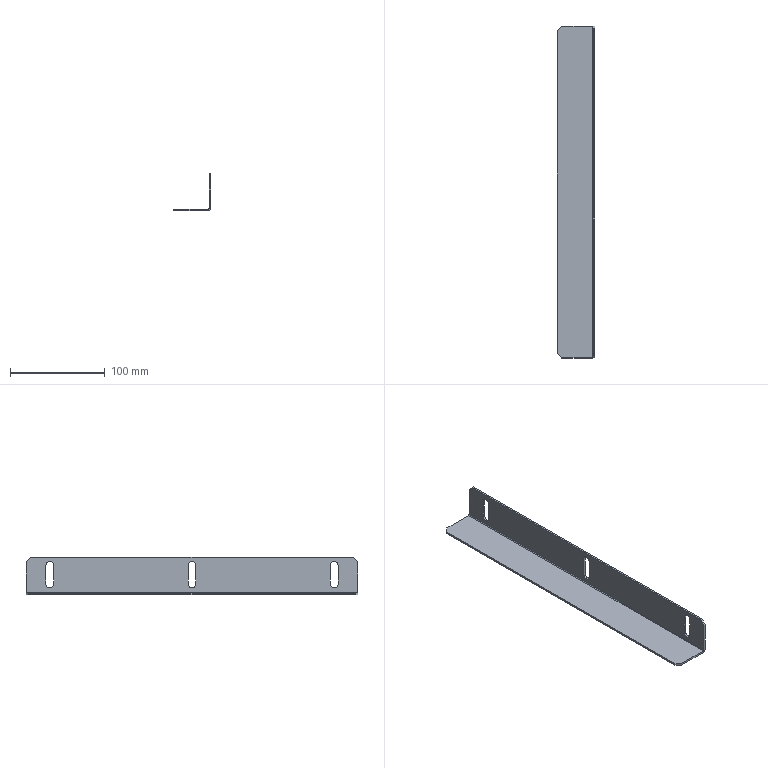Part | SolidWorks | features BreakCorner 1, EdgeFlange 1, FlatPattern 1, HoleWzd 1, SMBaseFlange 1, SheetMetal 1 | 1 solid | 33 faces | box 40 x 350 x 40 mm | volume 52717 mm3 | plane 22 | cylinder 11 | commonest cylinder face diameters 8 x9 1.473 x1 5.473 x1
STEP:
#1=CARTESIAN_POINT('',(20.,154.,29.368));
#2=VERTEX_POINT('',#1);
#3=CARTESIAN_POINT('',(20.,150.,33.368));
#4=VERTEX_POINT('',#3);
#5=CARTESIAN_POINT('',(20.,150.,29.368));
#6=DIRECTION('',(1.,0.,0.));
#7=DIRECTION('',(0.,0.,-1.));
#8=AXIS2_PLACEMENT_3D('',#5,#6,#7);
#9=CIRCLE('',#8,4.);
#10=EDGE_CURVE('',#2,#4,#9,.T.);
#11=ORIENTED_EDGE('',*,*,#10,.T.);
#12=CARTESIAN_POINT('',(18.,150.,33.368));
#13=VERTEX_POINT('',#12);
#14=CARTESIAN_POINT('',(18.,150.,33.368));
#15=DIRECTION('',(-1.,0.,0.));
#16=VECTOR('',#15,1000.);
#17=LINE('',#14,#16);
#18=EDGE_CURVE('',#4,#13,#17,.T.);
#19=ORIENTED_EDGE('',*,*,#18,.T.);
#20=CARTESIAN_POINT('',(18.,154.,29.368));
#21=VERTEX_POINT('',#20);
#22=CARTESIAN_POINT('',(18.,150.,29.368));
#23=DIRECTION('',(-1.,0.,0.));
#24=DIRECTION('',(0.,0.,1.));
#25=AXIS2_PLACEMENT_3D('',#22,#23,#24);
#26=CIRCLE('',#25,4.);
#27=EDGE_CURVE('',#13,#21,#26,.T.);
#28=ORIENTED_EDGE('',*,*,#27,.T.);
#29=CARTESIAN_POINT('',(20.001,154.,29.368));
#30=DIRECTION('',(1.,0.,0.));
#31=VECTOR('',#30,1000.);
#32=LINE('',#29,#31);
#33=EDGE_CURVE('',#21,#2,#32,.T.);
#34=ORIENTED_EDGE('',*,*,#33,.T.);
#35=EDGE_LOOP('',(#11,#19,#28,#34));
#36=FACE_OUTER_BOUND('',#35,.T.);
#37=CARTESIAN_POINT('',(18.,150.,29.368));
#38=DIRECTION('',(-1.,0.,0.));
#39=DIRECTION('',(0.,0.,1.));
#40=AXIS2_PLACEMENT_3D('',#37,#38,#39);
#41=CYLINDRICAL_SURFACE('',#40,4.);
#42=ADVANCED_FACE('',(#36),#41,.F.);
#43=CARTESIAN_POINT('',(20.,4.,29.368));
#44=VERTEX_POINT('',#43);
#45=CARTESIAN_POINT('',(20.,0.,33.368));
#46=VERTEX_POINT('',#45);
#47=CARTESIAN_POINT('',(20.,0.,29.368));
#48=DIRECTION('',(1.,0.,0.));
#49=DIRECTION('',(0.,0.,-1.));
#50=AXIS2_PLACEMENT_3D('',#47,#48,#49);
#51=CIRCLE('',#50,4.);
#52=EDGE_CURVE('',#44,#46,#51,.T.);
#53=ORIENTED_EDGE('',*,*,#52,.T.);
#54=CARTESIAN_POINT('',(18.,0.,33.368));
#55=VERTEX_POINT('',#54);
#56=CARTESIAN_POINT('',(18.,0.,33.368));
#57=DIRECTION('',(-1.,0.,0.));
#58=VECTOR('',#57,1000.);
#59=LINE('',#56,#58);
#60=EDGE_CURVE('',#46,#55,#59,.T.);
#61=ORIENTED_EDGE('',*,*,#60,.T.);
#62=CARTESIAN_POINT('',(18.,4.,29.368));
#63=VERTEX_POINT('',#62);
#64=CARTESIAN_POINT('',(18.,0.,29.368));
#65=DIRECTION('',(-1.,0.,0.));
#66=DIRECTION('',(0.,0.,1.));
#67=AXIS2_PLACEMENT_3D('',#64,#65,#66);
#68=CIRCLE('',#67,4.);
#69=EDGE_CURVE('',#55,#63,#68,.T.);
#70=ORIENTED_EDGE('',*,*,#69,.T.);
#71=CARTESIAN_POINT('',(20.001,4.,29.368));
#72=DIRECTION('',(1.,0.,0.));
#73=VECTOR('',#72,1000.);
#74=LINE('',#71,#73);
#75=EDGE_CURVE('',#63,#44,#74,.T.);
#76=ORIENTED_EDGE('',*,*,#75,.T.);
#77=EDGE_LOOP('',(#53,#61,#70,#76));
#78=FACE_OUTER_BOUND('',#77,.T.);
#79=CARTESIAN_POINT('',(18.,0.,29.368));
#80=DIRECTION('',(-1.,0.,0.));
#81=DIRECTION('',(0.,0.,1.));
#82=AXIS2_PLACEMENT_3D('',#79,#80,#81);
#83=CYLINDRICAL_SURFACE('',#82,4.);
#84=ADVANCED_FACE('',(#78),#83,.F.);
#85=CARTESIAN_POINT('',(20.,-146.,29.368));
#86=VERTEX_POINT('',#85);
#87=CARTESIAN_POINT('',(20.,-150.,33.368));
#88=VERTEX_POINT('',#87);
#89=CARTESIAN_POINT('',(20.,-150.,29.368));
#90=DIRECTION('',(1.,0.,0.));
#91=DIRECTION('',(0.,0.,-1.));
#92=AXIS2_PLACEMENT_3D('',#89,#90,#91);
#93=CIRCLE('',#92,4.);
#94=EDGE_CURVE('',#86,#88,#93,.T.);
#95=ORIENTED_EDGE('',*,*,#94,.T.);
#96=CARTESIAN_POINT('',(18.,-150.,33.368));
#97=VERTEX_POINT('',#96);
#98=CARTESIAN_POINT('',(18.,-150.,33.368));
#99=DIRECTION('',(-1.,0.,0.));
#100=VECTOR('',#99,1000.);
#101=LINE('',#98,#100);
#102=EDGE_CURVE('',#88,#97,#101,.T.);
#103=ORIENTED_EDGE('',*,*,#102,.T.);
#104=CARTESIAN_POINT('',(18.,-146.,29.368));
#105=VERTEX_POINT('',#104);
#106=CARTESIAN_POINT('',(18.,-150.,29.368));
#107=DIRECTION('',(-1.,0.,0.));
#108=DIRECTION('',(0.,0.,1.));
#109=AXIS2_PLACEMENT_3D('',#106,#107,#108);
#110=CIRCLE('',#109,4.);
#111=EDGE_CURVE('',#97,#105,#110,.T.);
#112=ORIENTED_EDGE('',*,*,#111,.T.);
#113=CARTESIAN_POINT('',(20.001,-146.,29.368));
#114=DIRECTION('',(1.,0.,0.));
#115=VECTOR('',#114,1000.);
#116=LINE('',#113,#115);
#117=EDGE_CURVE('',#105,#86,#116,.T.);
#118=ORIENTED_EDGE('',*,*,#117,.T.);
#119=EDGE_LOOP('',(#95,#103,#112,#118));
#120=FACE_OUTER_BOUND('',#119,.T.);
#121=CARTESIAN_POINT('',(18.,-150.,29.368));
#122=DIRECTION('',(-1.,0.,0.));
#123=DIRECTION('',(0.,0.,1.));
#124=AXIS2_PLACEMENT_3D('',#121,#122,#123);
#125=CYLINDRICAL_SURFACE('',#124,4.);
#126=ADVANCED_FACE('',(#120),#125,.F.);
#127=CARTESIAN_POINT('',(20.,175.,33.));
#128=VERTEX_POINT('',#127);
#129=CARTESIAN_POINT('',(20.,175.,0.7366));
#130=VERTEX_POINT('',#129);
#131=CARTESIAN_POINT('',(20.,175.,0.));
#132=DIRECTION('',(0.,0.,-1.));
#133=VECTOR('',#132,1000.);
#134=LINE('',#131,#133);
#135=EDGE_CURVE('',#128,#130,#134,.T.);
#136=ORIENTED_EDGE('',*,*,#135,.F.);
#137=CARTESIAN_POINT('',(20.,170.,38.));
#138=VERTEX_POINT('',#137);
#139=CARTESIAN_POINT('',(20.,104.,104.));
#140=DIRECTION('',(0.,-0.7071,0.7071));
#141=VECTOR('',#140,1000.);
#142=LINE('',#139,#141);
#143=EDGE_CURVE('',#128,#138,#142,.T.);
#144=ORIENTED_EDGE('',*,*,#143,.T.);
#145=CARTESIAN_POINT('',(20.,-170.,38.));
#146=VERTEX_POINT('',#145);
#147=CARTESIAN_POINT('',(20.,175.,38.));
#148=DIRECTION('',(0.,1.,0.));
#149=VECTOR('',#148,1000.);
#150=LINE('',#147,#149);
#151=EDGE_CURVE('',#146,#138,#150,.T.);
#152=ORIENTED_EDGE('',*,*,#151,.F.);
#153=CARTESIAN_POINT('',(20.,-175.,33.));
#154=VERTEX_POINT('',#153);
#155=CARTESIAN_POINT('',(20.,-104.,104.));
#156=DIRECTION('',(0.,-0.7071,-0.7071));
#157=VECTOR('',#156,1000.);
#158=LINE('',#155,#157);
#159=EDGE_CURVE('',#146,#154,#158,.T.);
#160=ORIENTED_EDGE('',*,*,#159,.T.);
#161=CARTESIAN_POINT('',(20.,-175.,0.7366));
#162=VERTEX_POINT('',#161);
#163=CARTESIAN_POINT('',(20.,-175.,38.));
#164=DIRECTION('',(0.,0.,1.));
#165=VECTOR('',#164,1000.);
#166=LINE('',#163,#165);
#167=EDGE_CURVE('',#162,#154,#166,.T.);
#168=ORIENTED_EDGE('',*,*,#167,.F.);
#169=CARTESIAN_POINT('',(20.,0.,0.7366));
#170=DIRECTION('',(0.,1.,0.));
#171=VECTOR('',#170,1000.);
#172=LINE('',#169,#171);
#173=EDGE_CURVE('',#162,#130,#172,.T.);
#174=ORIENTED_EDGE('',*,*,#173,.T.);
#175=EDGE_LOOP('',(#136,#144,#152,#160,#168,#174));
#176=FACE_OUTER_BOUND('',#175,.T.);
#177=ORIENTED_EDGE('',*,*,#94,.F.);
#178=CARTESIAN_POINT('',(20.,-146.,9.368));
#179=VERTEX_POINT('',#178);
#180=CARTESIAN_POINT('',(20.,-146.,0.));
#181=DIRECTION('',(0.,0.,-1.));
#182=VECTOR('',#181,1000.);
#183=LINE('',#180,#182);
#184=EDGE_CURVE('',#86,#179,#183,.T.);
#185=ORIENTED_EDGE('',*,*,#184,.T.);
#186=CARTESIAN_POINT('',(20.,-154.,9.368));
#187=VERTEX_POINT('',#186);
#188=CARTESIAN_POINT('',(20.,-150.,9.368));
#189=DIRECTION('',(1.,0.,0.));
#190=DIRECTION('',(0.,0.,-1.));
#191=AXIS2_PLACEMENT_3D('',#188,#189,#190);
#192=CIRCLE('',#191,4.);
#193=EDGE_CURVE('',#187,#179,#192,.T.);
#194=ORIENTED_EDGE('',*,*,#193,.F.);
#195=CARTESIAN_POINT('',(20.,-154.,29.368));
#196=VERTEX_POINT('',#195);
#197=CARTESIAN_POINT('',(20.,-154.,0.));
#198=DIRECTION('',(0.,0.,-1.));
#199=VECTOR('',#198,1000.);
#200=LINE('',#197,#199);
#201=EDGE_CURVE('',#196,#187,#200,.T.);
#202=ORIENTED_EDGE('',*,*,#201,.F.);
#203=CARTESIAN_POINT('',(20.,-150.,29.368));
#204=DIRECTION('',(1.,0.,0.));
#205=DIRECTION('',(0.,0.,-1.));
#206=AXIS2_PLACEMENT_3D('',#203,#204,#205);
#207=CIRCLE('',#206,4.);
#208=EDGE_CURVE('',#88,#196,#207,.T.);
#209=ORIENTED_EDGE('',*,*,#208,.F.);
#210=EDGE_LOOP('',(#177,#185,#194,#202,#209));
#211=FACE_BOUND('',#210,.T.);
#212=ORIENTED_EDGE('',*,*,#52,.F.);
#213=CARTESIAN_POINT('',(20.,4.,9.368));
#214=VERTEX_POINT('',#213);
#215=CARTESIAN_POINT('',(20.,4.,0.));
#216=DIRECTION('',(0.,0.,-1.));
#217=VECTOR('',#216,1000.);
#218=LINE('',#215,#217);
#219=EDGE_CURVE('',#44,#214,#218,.T.);
#220=ORIENTED_EDGE('',*,*,#219,.T.);
#221=CARTESIAN_POINT('',(20.,-4.,9.368));
#222=VERTEX_POINT('',#221);
#223=CARTESIAN_POINT('',(20.,0.,9.368));
#224=DIRECTION('',(1.,0.,0.));
#225=DIRECTION('',(0.,0.,-1.));
#226=AXIS2_PLACEMENT_3D('',#223,#224,#225);
#227=CIRCLE('',#226,4.);
#228=EDGE_CURVE('',#222,#214,#227,.T.);
#229=ORIENTED_EDGE('',*,*,#228,.F.);
#230=CARTESIAN_POINT('',(20.,-4.,29.368));
#231=VERTEX_POINT('',#230);
#232=CARTESIAN_POINT('',(20.,-4.,0.));
#233=DIRECTION('',(0.,0.,-1.));
#234=VECTOR('',#233,1000.);
#235=LINE('',#232,#234);
#236=EDGE_CURVE('',#231,#222,#235,.T.);
#237=ORIENTED_EDGE('',*,*,#236,.F.);
#238=CARTESIAN_POINT('',(20.,0.,29.368));
#239=DIRECTION('',(1.,0.,0.));
#240=DIRECTION('',(0.,0.,-1.));
#241=AXIS2_PLACEMENT_3D('',#238,#239,#240);
#242=CIRCLE('',#241,4.);
#243=EDGE_CURVE('',#46,#231,#242,.T.);
#244=ORIENTED_EDGE('',*,*,#243,.F.);
#245=EDGE_LOOP('',(#212,#220,#229,#237,#244));
#246=FACE_BOUND('',#245,.T.);
#247=ORIENTED_EDGE('',*,*,#10,.F.);
#248=CARTESIAN_POINT('',(20.,154.,9.368));
#249=VERTEX_POINT('',#248);
#250=CARTESIAN_POINT('',(20.,154.,0.));
#251=DIRECTION('',(0.,0.,-1.));
#252=VECTOR('',#251,1000.);
#253=LINE('',#250,#252);
#254=EDGE_CURVE('',#2,#249,#253,.T.);
#255=ORIENTED_EDGE('',*,*,#254,.T.);
#256=CARTESIAN_POINT('',(20.,146.,9.368));
#257=VERTEX_POINT('',#256);
#258=CARTESIAN_POINT('',(20.,150.,9.368));
#259=DIRECTION('',(1.,0.,0.));
#260=DIRECTION('',(0.,0.,-1.));
#261=AXIS2_PLACEMENT_3D('',#258,#259,#260);
#262=CIRCLE('',#261,4.);
#263=EDGE_CURVE('',#257,#249,#262,.T.);
#264=ORIENTED_EDGE('',*,*,#263,.F.);
#265=CARTESIAN_POINT('',(20.,146.,29.368));
#266=VERTEX_POINT('',#265);
#267=CARTESIAN_POINT('',(20.,146.,0.));
#268=DIRECTION('',(0.,0.,-1.));
#269=VECTOR('',#268,1000.);
#270=LINE('',#267,#269);
#271=EDGE_CURVE('',#266,#257,#270,.T.);
#272=ORIENTED_EDGE('',*,*,#271,.F.);
#273=CARTESIAN_POINT('',(20.,150.,29.368));
#274=DIRECTION('',(1.,0.,0.));
#275=DIRECTION('',(0.,0.,-1.));
#276=AXIS2_PLACEMENT_3D('',#273,#274,#275);
#277=CIRCLE('',#276,4.);
#278=EDGE_CURVE('',#4,#266,#277,.T.);
#279=ORIENTED_EDGE('',*,*,#278,.F.);
#280=EDGE_LOOP('',(#247,#255,#264,#272,#279));
#281=FACE_BOUND('',#280,.T.);
#282=CARTESIAN_POINT('',(20.,0.,0.));
#283=DIRECTION('',(1.,0.,0.));
#284=DIRECTION('',(0.,0.,-1.));
#285=AXIS2_PLACEMENT_3D('',#282,#283,#284);
#286=PLANE('',#285);
#287=ADVANCED_FACE('',(#176,#211,#246,#281),#286,.T.);
#288=CARTESIAN_POINT('',(18.,154.,9.368));
#289=VERTEX_POINT('',#288);
#290=CARTESIAN_POINT('',(18.,154.,9.368));
#291=DIRECTION('',(0.,0.,1.));
#292=VECTOR('',#291,1000.);
#293=LINE('',#290,#292);
#294=EDGE_CURVE('',#289,#21,#293,.T.);
#295=ORIENTED_EDGE('',*,*,#294,.T.);
#296=ORIENTED_EDGE('',*,*,#27,.F.);
#297=CARTESIAN_POINT('',(18.,146.,29.368));
#298=VERTEX_POINT('',#297);
#299=CARTESIAN_POINT('',(18.,150.,29.368));
#300=DIRECTION('',(-1.,0.,0.));
#301=DIRECTION('',(0.,0.,1.));
#302=AXIS2_PLACEMENT_3D('',#299,#300,#301);
#303=CIRCLE('',#302,4.);
#304=EDGE_CURVE('',#298,#13,#303,.T.);
#305=ORIENTED_EDGE('',*,*,#304,.F.);
#306=CARTESIAN_POINT('',(18.,146.,9.368));
#307=VERTEX_POINT('',#306);
#308=CARTESIAN_POINT('',(18.,146.,9.368));
#309=DIRECTION('',(0.,0.,1.));
#310=VECTOR('',#309,1000.);
#311=LINE('',#308,#310);
#312=EDGE_CURVE('',#307,#298,#311,.T.);
#313=ORIENTED_EDGE('',*,*,#312,.F.);
#314=CARTESIAN_POINT('',(18.,150.,9.368));
#315=DIRECTION('',(-1.,0.,0.));
#316=DIRECTION('',(0.,0.,1.));
#317=AXIS2_PLACEMENT_3D('',#314,#315,#316);
#318=CIRCLE('',#317,4.);
#319=EDGE_CURVE('',#289,#307,#318,.T.);
#320=ORIENTED_EDGE('',*,*,#319,.F.);
#321=EDGE_LOOP('',(#295,#296,#305,#313,#320));
#322=FACE_BOUND('',#321,.T.);
#323=CARTESIAN_POINT('',(18.,-154.,9.368));
#324=VERTEX_POINT('',#323);
#325=CARTESIAN_POINT('',(18.,-154.,29.368));
#326=VERTEX_POINT('',#325);
#327=CARTESIAN_POINT('',(18.,-154.,9.368));
#328=DIRECTION('',(0.,0.,1.));
#329=VECTOR('',#328,1000.);
#330=LINE('',#327,#329);
#331=EDGE_CURVE('',#324,#326,#330,.T.);
#332=ORIENTED_EDGE('',*,*,#331,.F.);
#333=CARTESIAN_POINT('',(18.,-146.,9.368));
#334=VERTEX_POINT('',#333);
#335=CARTESIAN_POINT('',(18.,-150.,9.368));
#336=DIRECTION('',(-1.,0.,0.));
#337=DIRECTION('',(0.,0.,1.));
#338=AXIS2_PLACEMENT_3D('',#335,#336,#337);
#339=CIRCLE('',#338,4.);
#340=EDGE_CURVE('',#334,#324,#339,.T.);
#341=ORIENTED_EDGE('',*,*,#340,.F.);
#342=CARTESIAN_POINT('',(18.,-146.,9.368));
#343=DIRECTION('',(0.,0.,1.));
#344=VECTOR('',#343,1000.);
#345=LINE('',#342,#344);
#346=EDGE_CURVE('',#334,#105,#345,.T.);
#347=ORIENTED_EDGE('',*,*,#346,.T.);
#348=ORIENTED_EDGE('',*,*,#111,.F.);
#349=CARTESIAN_POINT('',(18.,-150.,29.368));
#350=DIRECTION('',(-1.,0.,0.));
#351=DIRECTION('',(0.,0.,1.));
#352=AXIS2_PLACEMENT_3D('',#349,#350,#351);
#353=CIRCLE('',#352,4.);
#354=EDGE_CURVE('',#326,#97,#353,.T.);
#355=ORIENTED_EDGE('',*,*,#354,.F.);
#356=EDGE_LOOP('',(#332,#341,#347,#348,#355));
#357=FACE_BOUND('',#356,.T.);
#358=CARTESIAN_POINT('',(18.,-170.,38.));
#359=VERTEX_POINT('',#358);
#360=CARTESIAN_POINT('',(18.,170.,38.));
#361=VERTEX_POINT('',#360);
#362=CARTESIAN_POINT('',(18.,0.,38.));
#363=DIRECTION('',(0.,1.,0.));
#364=VECTOR('',#363,1000.);
#365=LINE('',#362,#364);
#366=EDGE_CURVE('',#359,#361,#365,.T.);
#367=ORIENTED_EDGE('',*,*,#366,.T.);
#368=CARTESIAN_POINT('',(18.,175.,33.));
#369=VERTEX_POINT('',#368);
#370=CARTESIAN_POINT('',(18.,170.,38.));
#371=DIRECTION('',(0.,0.7071,-0.7071));
#372=VECTOR('',#371,1000.);
#373=LINE('',#370,#372);
#374=EDGE_CURVE('',#361,#369,#373,.T.);
#375=ORIENTED_EDGE('',*,*,#374,.T.);
#376=CARTESIAN_POINT('',(18.,175.,0.7366));
#377=VERTEX_POINT('',#376);
#378=CARTESIAN_POINT('',(18.,175.,0.));
#379=DIRECTION('',(0.,0.,-1.));
#380=VECTOR('',#379,1000.);
#381=LINE('',#378,#380);
#382=EDGE_CURVE('',#369,#377,#381,.T.);
#383=ORIENTED_EDGE('',*,*,#382,.T.);
#384=CARTESIAN_POINT('',(18.,-175.,0.7366));
#385=VERTEX_POINT('',#384);
#386=CARTESIAN_POINT('',(18.,-175.,0.7366));
#387=DIRECTION('',(0.,1.,0.));
#388=VECTOR('',#387,1000.);
#389=LINE('',#386,#388);
#390=EDGE_CURVE('',#385,#377,#389,.T.);
#391=ORIENTED_EDGE('',*,*,#390,.F.);
#392=CARTESIAN_POINT('',(18.,-175.,33.));
#393=VERTEX_POINT('',#392);
#394=CARTESIAN_POINT('',(18.,-175.,0.));
#395=DIRECTION('',(0.,0.,1.));
#396=VECTOR('',#395,1000.);
#397=LINE('',#394,#396);
#398=EDGE_CURVE('',#385,#393,#397,.T.);
#399=ORIENTED_EDGE('',*,*,#398,.T.);
#400=CARTESIAN_POINT('',(18.,-175.,33.));
#401=DIRECTION('',(0.,0.7071,0.7071));
#402=VECTOR('',#401,1000.);
#403=LINE('',#400,#402);
#404=EDGE_CURVE('',#393,#359,#403,.T.);
#405=ORIENTED_EDGE('',*,*,#404,.T.);
#406=EDGE_LOOP('',(#367,#375,#383,#391,#399,#405));
#407=FACE_OUTER_BOUND('',#406,.T.);
#408=CARTESIAN_POINT('',(18.,-4.,9.368));
#409=VERTEX_POINT('',#408);
#410=CARTESIAN_POINT('',(18.,-4.,29.368));
#411=VERTEX_POINT('',#410);
#412=CARTESIAN_POINT('',(18.,-4.,9.368));
#413=DIRECTION('',(0.,0.,1.));
#414=VECTOR('',#413,1000.);
#415=LINE('',#412,#414);
#416=EDGE_CURVE('',#409,#411,#415,.T.);
#417=ORIENTED_EDGE('',*,*,#416,.F.);
#418=CARTESIAN_POINT('',(18.,4.,9.368));
#419=VERTEX_POINT('',#418);
#420=CARTESIAN_POINT('',(18.,0.,9.368));
#421=DIRECTION('',(-1.,0.,0.));
#422=DIRECTION('',(0.,0.,1.));
#423=AXIS2_PLACEMENT_3D('',#420,#421,#422);
#424=CIRCLE('',#423,4.);
#425=EDGE_CURVE('',#419,#409,#424,.T.);
#426=ORIENTED_EDGE('',*,*,#425,.F.);
#427=CARTESIAN_POINT('',(18.,4.,9.368));
#428=DIRECTION('',(0.,0.,1.));
#429=VECTOR('',#428,1000.);
#430=LINE('',#427,#429);
#431=EDGE_CURVE('',#419,#63,#430,.T.);
#432=ORIENTED_EDGE('',*,*,#431,.T.);
#433=ORIENTED_EDGE('',*,*,#69,.F.);
#434=CARTESIAN_POINT('',(18.,0.,29.368));
#435=DIRECTION('',(-1.,0.,0.));
#436=DIRECTION('',(0.,0.,1.));
#437=AXIS2_PLACEMENT_3D('',#434,#435,#436);
#438=CIRCLE('',#437,4.);
#439=EDGE_CURVE('',#411,#55,#438,.T.);
#440=ORIENTED_EDGE('',*,*,#439,.F.);
#441=EDGE_LOOP('',(#417,#426,#432,#433,#440));
#442=FACE_BOUND('',#441,.T.);
#443=CARTESIAN_POINT('',(18.,0.,0.));
#444=DIRECTION('',(1.,0.,0.));
#445=DIRECTION('',(0.,0.,-1.));
#446=AXIS2_PLACEMENT_3D('',#443,#444,#445);
#447=PLANE('',#446);
#448=ADVANCED_FACE('',(#322,#357,#407,#442),#447,.F.);
#449=CARTESIAN_POINT('',(17.263,175.,-2.));
#450=VERTEX_POINT('',#449);
#451=CARTESIAN_POINT('',(-15.,175.,-2.));
#452=VERTEX_POINT('',#451);
#453=CARTESIAN_POINT('',(-20.,175.,-2.));
#454=DIRECTION('',(-1.,0.,0.));
#455=VECTOR('',#454,1000.);
#456=LINE('',#453,#455);
#457=EDGE_CURVE('',#450,#452,#456,.T.);
#458=ORIENTED_EDGE('',*,*,#457,.T.);
#459=CARTESIAN_POINT('',(-15.,175.,0.));
#460=VERTEX_POINT('',#459);
#461=CARTESIAN_POINT('',(-15.,175.,-2.));
#462=DIRECTION('',(0.,0.,1.));
#463=VECTOR('',#462,1000.);
#464=LINE('',#461,#463);
#465=EDGE_CURVE('',#452,#460,#464,.T.);
#466=ORIENTED_EDGE('',*,*,#465,.T.);
#467=CARTESIAN_POINT('',(17.263,175.,0.));
#468=VERTEX_POINT('',#467);
#469=CARTESIAN_POINT('',(-20.,175.,0.));
#470=DIRECTION('',(-1.,0.,0.));
#471=VECTOR('',#470,1000.);
#472=LINE('',#469,#471);
#473=EDGE_CURVE('',#468,#460,#472,.T.);
#474=ORIENTED_EDGE('',*,*,#473,.F.);
#475=CARTESIAN_POINT('',(17.263,175.,0.));
#476=DIRECTION('',(0.,0.,-1.));
#477=VECTOR('',#476,1000.);
#478=LINE('',#475,#477);
#479=EDGE_CURVE('',#468,#450,#478,.T.);
#480=ORIENTED_EDGE('',*,*,#479,.T.);
#481=EDGE_LOOP('',(#458,#466,#474,#480));
#482=FACE_OUTER_BOUND('',#481,.T.);
#483=CARTESIAN_POINT('',(-20.,175.,-2.));
#484=DIRECTION('',(0.,1.,0.));
#485=DIRECTION('',(0.,0.,1.));
#486=AXIS2_PLACEMENT_3D('',#483,#484,#485);
#487=PLANE('',#486);
#488=ADVANCED_FACE('',(#482),#487,.T.);
#489=CARTESIAN_POINT('',(-15.,-175.,-2.));
#490=VERTEX_POINT('',#489);
#491=CARTESIAN_POINT('',(17.263,-175.,-2.));
#492=VERTEX_POINT('',#491);
#493=CARTESIAN_POINT('',(-20.,-175.,-2.));
#494=DIRECTION('',(1.,0.,0.));
#495=VECTOR('',#494,1000.);
#496=LINE('',#493,#495);
#497=EDGE_CURVE('',#490,#492,#496,.T.);
#498=ORIENTED_EDGE('',*,*,#497,.F.);
#499=CARTESIAN_POINT('',(-20.,-170.,-2.));
#500=VERTEX_POINT('',#499);
#501=CARTESIAN_POINT('',(-95.,-95.,-2.));
#502=DIRECTION('',(-0.7071,0.7071,0.));
#503=VECTOR('',#502,1000.);
#504=LINE('',#501,#503);
#505=EDGE_CURVE('',#490,#500,#504,.T.);
#506=ORIENTED_EDGE('',*,*,#505,.T.);
#507=CARTESIAN_POINT('',(-20.,170.,-2.));
#508=VERTEX_POINT('',#507);
#509=CARTESIAN_POINT('',(-20.,-175.,-2.));
#510=DIRECTION('',(0.,-1.,0.));
#511=VECTOR('',#510,1000.);
#512=LINE('',#509,#511);
#513=EDGE_CURVE('',#508,#500,#512,.T.);
#514=ORIENTED_EDGE('',*,*,#513,.F.);
#515=CARTESIAN_POINT('',(-95.,95.,-2.));
#516=DIRECTION('',(0.7071,0.7071,0.));
#517=VECTOR('',#516,1000.);
#518=LINE('',#515,#517);
#519=EDGE_CURVE('',#508,#452,#518,.T.);
#520=ORIENTED_EDGE('',*,*,#519,.T.);
#521=ORIENTED_EDGE('',*,*,#457,.F.);
#522=CARTESIAN_POINT('',(17.263,175.,-2.));
#523=DIRECTION('',(0.,-1.,0.));
#524=VECTOR('',#523,1000.);
#525=LINE('',#522,#524);
#526=EDGE_CURVE('',#450,#492,#525,.T.);
#527=ORIENTED_EDGE('',*,*,#526,.T.);
#528=EDGE_LOOP('',(#498,#506,#514,#520,#521,#527));
#529=FACE_OUTER_BOUND('',#528,.T.);
#530=CARTESIAN_POINT('',(0.,0.,-2.));
#531=DIRECTION('',(0.,0.,-1.));
#532=DIRECTION('',(-1.,0.,0.));
#533=AXIS2_PLACEMENT_3D('',#530,#531,#532);
#534=PLANE('',#533);
#535=ADVANCED_FACE('',(#529),#534,.T.);
#536=CARTESIAN_POINT('',(-20.,170.,0.));
#537=VERTEX_POINT('',#536);
#538=CARTESIAN_POINT('',(-20.,-170.,0.));
#539=VERTEX_POINT('',#538);
#540=CARTESIAN_POINT('',(-20.,-175.,0.));
#541=DIRECTION('',(0.,-1.,0.));
#542=VECTOR('',#541,1000.);
#543=LINE('',#540,#542);
#544=EDGE_CURVE('',#537,#539,#543,.T.);
#545=ORIENTED_EDGE('',*,*,#544,.T.);
#546=CARTESIAN_POINT('',(-15.,-175.,0.));
#547=VERTEX_POINT('',#546);
#548=CARTESIAN_POINT('',(-20.,-170.,0.));
#549=DIRECTION('',(0.7071,-0.7071,0.));
#550=VECTOR('',#549,1000.);
#551=LINE('',#548,#550);
#552=EDGE_CURVE('',#539,#547,#551,.T.);
#553=ORIENTED_EDGE('',*,*,#552,.T.);
#554=CARTESIAN_POINT('',(17.263,-175.,0.));
#555=VERTEX_POINT('',#554);
#556=CARTESIAN_POINT('',(-20.,-175.,0.));
#557=DIRECTION('',(1.,0.,0.));
#558=VECTOR('',#557,1000.);
#559=LINE('',#556,#558);
#560=EDGE_CURVE('',#547,#555,#559,.T.);
#561=ORIENTED_EDGE('',*,*,#560,.T.);
#562=CARTESIAN_POINT('',(17.263,175.,0.));
#563=DIRECTION('',(0.,-1.,0.));
#564=VECTOR('',#563,1000.);
#565=LINE('',#562,#564);
#566=EDGE_CURVE('',#468,#555,#565,.T.);
#567=ORIENTED_EDGE('',*,*,#566,.F.);
#568=ORIENTED_EDGE('',*,*,#473,.T.);
#569=CARTESIAN_POINT('',(-15.,175.,0.));
#570=DIRECTION('',(-0.7071,-0.7071,0.));
#571=VECTOR('',#570,1000.);
#572=LINE('',#569,#571);
#573=EDGE_CURVE('',#460,#537,#572,.T.);
#574=ORIENTED_EDGE('',*,*,#573,.T.);
#575=EDGE_LOOP('',(#545,#553,#561,#567,#568,#574));
#576=FACE_OUTER_BOUND('',#575,.T.);
#577=CARTESIAN_POINT('',(0.,0.,0.));
#578=DIRECTION('',(0.,0.,-1.));
#579=DIRECTION('',(-1.,0.,0.));
#580=AXIS2_PLACEMENT_3D('',#577,#578,#579);
#581=PLANE('',#580);
#582=ADVANCED_FACE('',(#576),#581,.F.);
#583=ORIENTED_EDGE('',*,*,#560,.F.);
#584=CARTESIAN_POINT('',(-15.,-175.,-2.));
#585=DIRECTION('',(0.,0.,-1.));
#586=VECTOR('',#585,1000.);
#587=LINE('',#584,#586);
#588=EDGE_CURVE('',#547,#490,#587,.T.);
#589=ORIENTED_EDGE('',*,*,#588,.T.);
#590=ORIENTED_EDGE('',*,*,#497,.T.);
#591=CARTESIAN_POINT('',(17.263,-175.,0.));
#592=DIRECTION('',(0.,0.,-1.));
#593=VECTOR('',#592,1000.);
#594=LINE('',#591,#593);
#595=EDGE_CURVE('',#555,#492,#594,.T.);
#596=ORIENTED_EDGE('',*,*,#595,.F.);
#597=EDGE_LOOP('',(#583,#589,#590,#596));
#598=FACE_OUTER_BOUND('',#597,.T.);
#599=CARTESIAN_POINT('',(-20.,-175.,-2.));
#600=DIRECTION('',(0.,-1.,0.));
#601=DIRECTION('',(0.,0.,-1.));
#602=AXIS2_PLACEMENT_3D('',#599,#600,#601);
#603=PLANE('',#602);
#604=ADVANCED_FACE('',(#598),#603,.T.);
#605=ORIENTED_EDGE('',*,*,#513,.T.);
#606=CARTESIAN_POINT('',(-20.,-170.,-2.));
#607=DIRECTION('',(0.,0.,1.));
#608=VECTOR('',#607,1000.);
#609=LINE('',#606,#608);
#610=EDGE_CURVE('',#500,#539,#609,.T.);
#611=ORIENTED_EDGE('',*,*,#610,.T.);
#612=ORIENTED_EDGE('',*,*,#544,.F.);
#613=CARTESIAN_POINT('',(-20.,170.,-2.));
#614=DIRECTION('',(0.,0.,-1.));
#615=VECTOR('',#614,1000.);
#616=LINE('',#613,#615);
#617=EDGE_CURVE('',#537,#508,#616,.T.);
#618=ORIENTED_EDGE('',*,*,#617,.T.);
#619=EDGE_LOOP('',(#605,#611,#612,#618));
#620=FACE_OUTER_BOUND('',#619,.T.);
#621=CARTESIAN_POINT('',(-20.,-175.,-2.));
#622=DIRECTION('',(-1.,0.,0.));
#623=DIRECTION('',(0.,0.,1.));
#624=AXIS2_PLACEMENT_3D('',#621,#622,#623);
#625=PLANE('',#624);
#626=ADVANCED_FACE('',(#620),#625,.T.);
#627=CARTESIAN_POINT('',(20.,-175.,0.7366));
#628=DIRECTION('',(1.,0.,0.));
#629=VECTOR('',#628,1000.);
#630=LINE('',#627,#629);
#631=EDGE_CURVE('',#385,#162,#630,.T.);
#632=ORIENTED_EDGE('',*,*,#631,.F.);
#633=CARTESIAN_POINT('',(17.263,-175.,0.7366));
#634=DIRECTION('',(0.,-1.,0.));
#635=DIRECTION('',(0.,0.,1.));
#636=AXIS2_PLACEMENT_3D('',#633,#634,#635);
#637=CIRCLE('',#636,0.7366);
#638=EDGE_CURVE('',#555,#385,#637,.T.);
#639=ORIENTED_EDGE('',*,*,#638,.F.);
#640=ORIENTED_EDGE('',*,*,#595,.T.);
#641=CARTESIAN_POINT('',(17.263,-175.,0.7366));
#642=DIRECTION('',(0.,-1.,0.));
#643=DIRECTION('',(0.,0.,1.));
#644=AXIS2_PLACEMENT_3D('',#641,#642,#643);
#645=CIRCLE('',#644,2.737);
#646=EDGE_CURVE('',#492,#162,#645,.T.);
#647=ORIENTED_EDGE('',*,*,#646,.T.);
#648=EDGE_LOOP('',(#632,#639,#640,#647));
#649=FACE_OUTER_BOUND('',#648,.T.);
#650=CARTESIAN_POINT('',(17.263,-175.,0.7366));
#651=DIRECTION('',(0.,-1.,0.));
#652=DIRECTION('',(0.,0.,-1.));
#653=AXIS2_PLACEMENT_3D('',#650,#651,#652);
#654=PLANE('',#653);
#655=ADVANCED_FACE('',(#649),#654,.T.);
#656=CARTESIAN_POINT('',(17.263,175.,0.7366));
#657=DIRECTION('',(0.,1.,0.));
#658=DIRECTION('',(0.,0.,1.));
#659=AXIS2_PLACEMENT_3D('',#656,#657,#658);
#660=CIRCLE('',#659,0.7366);
#661=EDGE_CURVE('',#377,#468,#660,.T.);
#662=ORIENTED_EDGE('',*,*,#661,.F.);
#663=CARTESIAN_POINT('',(18.,175.,0.7366));
#664=DIRECTION('',(1.,0.,0.));
#665=VECTOR('',#664,1000.);
#666=LINE('',#663,#665);
#667=EDGE_CURVE('',#377,#130,#666,.T.);
#668=ORIENTED_EDGE('',*,*,#667,.T.);
#669=CARTESIAN_POINT('',(17.263,175.,0.7366));
#670=DIRECTION('',(0.,1.,0.));
#671=DIRECTION('',(0.,0.,1.));
#672=AXIS2_PLACEMENT_3D('',#669,#670,#671);
#673=CIRCLE('',#672,2.737);
#674=EDGE_CURVE('',#130,#450,#673,.T.);
#675=ORIENTED_EDGE('',*,*,#674,.T.);
#676=ORIENTED_EDGE('',*,*,#479,.F.);
#677=EDGE_LOOP('',(#662,#668,#675,#676));
#678=FACE_OUTER_BOUND('',#677,.T.);
#679=CARTESIAN_POINT('',(17.263,175.,0.7366));
#680=DIRECTION('',(0.,-1.,0.));
#681=DIRECTION('',(0.,0.,-1.));
#682=AXIS2_PLACEMENT_3D('',#679,#680,#681);
#683=PLANE('',#682);
#684=ADVANCED_FACE('',(#678),#683,.F.);
#685=ORIENTED_EDGE('',*,*,#526,.F.);
#686=ORIENTED_EDGE('',*,*,#674,.F.);
#687=ORIENTED_EDGE('',*,*,#173,.F.);
#688=ORIENTED_EDGE('',*,*,#646,.F.);
#689=EDGE_LOOP('',(#685,#686,#687,#688));
#690=FACE_OUTER_BOUND('',#689,.T.);
#691=CARTESIAN_POINT('',(17.263,175.,0.7366));
#692=DIRECTION('',(0.,1.,0.));
#693=DIRECTION('',(1.,0.,0.));
#694=AXIS2_PLACEMENT_3D('',#691,#692,#693);
#695=CYLINDRICAL_SURFACE('',#694,2.737);
#696=ADVANCED_FACE('',(#690),#695,.T.);
#697=ORIENTED_EDGE('',*,*,#566,.T.);
#698=ORIENTED_EDGE('',*,*,#638,.T.);
#699=ORIENTED_EDGE('',*,*,#390,.T.);
#700=ORIENTED_EDGE('',*,*,#661,.T.);
#701=EDGE_LOOP('',(#697,#698,#699,#700));
#702=FACE_OUTER_BOUND('',#701,.T.);
#703=CARTESIAN_POINT('',(17.263,175.,0.7366));
#704=DIRECTION('',(0.,1.,0.));
#705=DIRECTION('',(1.,0.,0.));
#706=AXIS2_PLACEMENT_3D('',#703,#704,#705);
#707=CYLINDRICAL_SURFACE('',#706,0.7366);
#708=ADVANCED_FACE('',(#702),#707,.F.);
#709=ORIENTED_EDGE('',*,*,#382,.F.);
#710=CARTESIAN_POINT('',(20.,175.,33.));
#711=DIRECTION('',(1.,0.,0.));
#712=VECTOR('',#711,1000.);
#713=LINE('',#710,#712);
#714=EDGE_CURVE('',#369,#128,#713,.T.);
#715=ORIENTED_EDGE('',*,*,#714,.T.);
#716=ORIENTED_EDGE('',*,*,#135,.T.);
#717=ORIENTED_EDGE('',*,*,#667,.F.);
#718=EDGE_LOOP('',(#709,#715,#716,#717));
#719=FACE_OUTER_BOUND('',#718,.T.);
#720=CARTESIAN_POINT('',(20.,175.,0.));
#721=DIRECTION('',(0.,1.,0.));
#722=DIRECTION('',(0.,0.,1.));
#723=AXIS2_PLACEMENT_3D('',#720,#721,#722);
#724=PLANE('',#723);
#725=ADVANCED_FACE('',(#719),#724,.T.);
#726=ORIENTED_EDGE('',*,*,#167,.T.);
#727=CARTESIAN_POINT('',(20.,-175.,33.));
#728=DIRECTION('',(-1.,0.,0.));
#729=VECTOR('',#728,1000.);
#730=LINE('',#727,#729);
#731=EDGE_CURVE('',#154,#393,#730,.T.);
#732=ORIENTED_EDGE('',*,*,#731,.T.);
#733=ORIENTED_EDGE('',*,*,#398,.F.);
#734=ORIENTED_EDGE('',*,*,#631,.T.);
#735=EDGE_LOOP('',(#726,#732,#733,#734));
#736=FACE_OUTER_BOUND('',#735,.T.);
#737=CARTESIAN_POINT('',(20.,-175.,38.));
#738=DIRECTION('',(0.,-1.,0.));
#739=DIRECTION('',(0.,0.,-1.));
#740=AXIS2_PLACEMENT_3D('',#737,#738,#739);
#741=PLANE('',#740);
#742=ADVANCED_FACE('',(#736),#741,.T.);
#743=ORIENTED_EDGE('',*,*,#151,.T.);
#744=CARTESIAN_POINT('',(20.,170.,38.));
#745=DIRECTION('',(-1.,0.,0.));
#746=VECTOR('',#745,1000.);
#747=LINE('',#744,#746);
#748=EDGE_CURVE('',#138,#361,#747,.T.);
#749=ORIENTED_EDGE('',*,*,#748,.T.);
#750=ORIENTED_EDGE('',*,*,#366,.F.);
#751=CARTESIAN_POINT('',(20.,-170.,38.));
#752=DIRECTION('',(1.,0.,0.));
#753=VECTOR('',#752,1000.);
#754=LINE('',#751,#753);
#755=EDGE_CURVE('',#359,#146,#754,.T.);
#756=ORIENTED_EDGE('',*,*,#755,.T.);
#757=EDGE_LOOP('',(#743,#749,#750,#756));
#758=FACE_OUTER_BOUND('',#757,.T.);
#759=CARTESIAN_POINT('',(20.,175.,38.));
#760=DIRECTION('',(0.,0.,1.));
#761=DIRECTION('',(1.,0.,0.));
#762=AXIS2_PLACEMENT_3D('',#759,#760,#761);
#763=PLANE('',#762);
#764=ADVANCED_FACE('',(#758),#763,.T.);
#765=ORIENTED_EDGE('',*,*,#102,.F.);
#766=ORIENTED_EDGE('',*,*,#208,.T.);
#767=CARTESIAN_POINT('',(18.,-154.,29.368));
#768=DIRECTION('',(1.,0.,0.));
#769=VECTOR('',#768,1000.);
#770=LINE('',#767,#769);
#771=EDGE_CURVE('',#326,#196,#770,.T.);
#772=ORIENTED_EDGE('',*,*,#771,.F.);
#773=ORIENTED_EDGE('',*,*,#354,.T.);
#774=EDGE_LOOP('',(#765,#766,#772,#773));
#775=FACE_OUTER_BOUND('',#774,.T.);
#776=CARTESIAN_POINT('',(18.,-150.,29.368));
#777=DIRECTION('',(-1.,0.,0.));
#778=DIRECTION('',(0.,0.,1.));
#779=AXIS2_PLACEMENT_3D('',#776,#777,#778);
#780=CYLINDRICAL_SURFACE('',#779,4.);
#781=ADVANCED_FACE('',(#775),#780,.F.);
#782=ORIENTED_EDGE('',*,*,#193,.T.);
#783=CARTESIAN_POINT('',(20.001,-146.,9.368));
#784=DIRECTION('',(1.,0.,0.));
#785=VECTOR('',#784,1000.);
#786=LINE('',#783,#785);
#787=EDGE_CURVE('',#334,#179,#786,.T.);
#788=ORIENTED_EDGE('',*,*,#787,.F.);
#789=ORIENTED_EDGE('',*,*,#340,.T.);
#790=CARTESIAN_POINT('',(18.,-154.,9.368));
#791=DIRECTION('',(-1.,0.,0.));
#792=VECTOR('',#791,1000.);
#793=LINE('',#790,#792);
#794=EDGE_CURVE('',#187,#324,#793,.T.);
#795=ORIENTED_EDGE('',*,*,#794,.F.);
#796=EDGE_LOOP('',(#782,#788,#789,#795));
#797=FACE_OUTER_BOUND('',#796,.T.);
#798=CARTESIAN_POINT('',(18.,-150.,9.368));
#799=DIRECTION('',(-1.,0.,0.));
#800=DIRECTION('',(0.,0.,1.));
#801=AXIS2_PLACEMENT_3D('',#798,#799,#800);
#802=CYLINDRICAL_SURFACE('',#801,4.);
#803=ADVANCED_FACE('',(#797),#802,.F.);
#804=ORIENTED_EDGE('',*,*,#117,.F.);
#805=ORIENTED_EDGE('',*,*,#346,.F.);
#806=ORIENTED_EDGE('',*,*,#787,.T.);
#807=ORIENTED_EDGE('',*,*,#184,.F.);
#808=EDGE_LOOP('',(#804,#805,#806,#807));
#809=FACE_OUTER_BOUND('',#808,.T.);
#810=CARTESIAN_POINT('',(20.001,-146.,9.368));
#811=DIRECTION('',(0.,-1.,0.));
#812=DIRECTION('',(1.,0.,0.));
#813=AXIS2_PLACEMENT_3D('',#810,#811,#812);
#814=PLANE('',#813);
#815=ADVANCED_FACE('',(#809),#814,.T.);
#816=ORIENTED_EDGE('',*,*,#201,.T.);
#817=ORIENTED_EDGE('',*,*,#794,.T.);
#818=ORIENTED_EDGE('',*,*,#331,.T.);
#819=ORIENTED_EDGE('',*,*,#771,.T.);
#820=EDGE_LOOP('',(#816,#817,#818,#819));
#821=FACE_OUTER_BOUND('',#820,.T.);
#822=CARTESIAN_POINT('',(18.,-154.,9.368));
#823=DIRECTION('',(0.,-1.,0.));
#824=DIRECTION('',(0.,0.,-1.));
#825=AXIS2_PLACEMENT_3D('',#822,#823,#824);
#826=PLANE('',#825);
#827=ADVANCED_FACE('',(#821),#826,.F.);
#828=ORIENTED_EDGE('',*,*,#60,.F.);
#829=ORIENTED_EDGE('',*,*,#243,.T.);
#830=CARTESIAN_POINT('',(18.,-4.,29.368));
#831=DIRECTION('',(1.,0.,0.));
#832=VECTOR('',#831,1000.);
#833=LINE('',#830,#832);
#834=EDGE_CURVE('',#411,#231,#833,.T.);
#835=ORIENTED_EDGE('',*,*,#834,.F.);
#836=ORIENTED_EDGE('',*,*,#439,.T.);
#837=EDGE_LOOP('',(#828,#829,#835,#836));
#838=FACE_OUTER_BOUND('',#837,.T.);
#839=CARTESIAN_POINT('',(18.,0.,29.368));
#840=DIRECTION('',(-1.,0.,0.));
#841=DIRECTION('',(0.,0.,1.));
#842=AXIS2_PLACEMENT_3D('',#839,#840,#841);
#843=CYLINDRICAL_SURFACE('',#842,4.);
#844=ADVANCED_FACE('',(#838),#843,.F.);
#845=ORIENTED_EDGE('',*,*,#228,.T.);
#846=CARTESIAN_POINT('',(20.001,4.,9.368));
#847=DIRECTION('',(1.,0.,0.));
#848=VECTOR('',#847,1000.);
#849=LINE('',#846,#848);
#850=EDGE_CURVE('',#419,#214,#849,.T.);
#851=ORIENTED_EDGE('',*,*,#850,.F.);
#852=ORIENTED_EDGE('',*,*,#425,.T.);
#853=CARTESIAN_POINT('',(18.,-4.,9.368));
#854=DIRECTION('',(-1.,0.,0.));
#855=VECTOR('',#854,1000.);
#856=LINE('',#853,#855);
#857=EDGE_CURVE('',#222,#409,#856,.T.);
#858=ORIENTED_EDGE('',*,*,#857,.F.);
#859=EDGE_LOOP('',(#845,#851,#852,#858));
#860=FACE_OUTER_BOUND('',#859,.T.);
#861=CARTESIAN_POINT('',(18.,0.,9.368));
#862=DIRECTION('',(-1.,0.,0.));
#863=DIRECTION('',(0.,0.,1.));
#864=AXIS2_PLACEMENT_3D('',#861,#862,#863);
#865=CYLINDRICAL_SURFACE('',#864,4.);
#866=ADVANCED_FACE('',(#860),#865,.F.);
#867=ORIENTED_EDGE('',*,*,#75,.F.);
#868=ORIENTED_EDGE('',*,*,#431,.F.);
#869=ORIENTED_EDGE('',*,*,#850,.T.);
#870=ORIENTED_EDGE('',*,*,#219,.F.);
#871=EDGE_LOOP('',(#867,#868,#869,#870));
#872=FACE_OUTER_BOUND('',#871,.T.);
#873=CARTESIAN_POINT('',(20.001,4.,9.368));
#874=DIRECTION('',(0.,-1.,0.));
#875=DIRECTION('',(1.,0.,0.));
#876=AXIS2_PLACEMENT_3D('',#873,#874,#875);
#877=PLANE('',#876);
#878=ADVANCED_FACE('',(#872),#877,.T.);
#879=ORIENTED_EDGE('',*,*,#236,.T.);
#880=ORIENTED_EDGE('',*,*,#857,.T.);
#881=ORIENTED_EDGE('',*,*,#416,.T.);
#882=ORIENTED_EDGE('',*,*,#834,.T.);
#883=EDGE_LOOP('',(#879,#880,#881,#882));
#884=FACE_OUTER_BOUND('',#883,.T.);
#885=CARTESIAN_POINT('',(18.,-4.,9.368));
#886=DIRECTION('',(0.,-1.,0.));
#887=DIRECTION('',(0.,0.,-1.));
#888=AXIS2_PLACEMENT_3D('',#885,#886,#887);
#889=PLANE('',#888);
#890=ADVANCED_FACE('',(#884),#889,.F.);
#891=ORIENTED_EDGE('',*,*,#18,.F.);
#892=ORIENTED_EDGE('',*,*,#278,.T.);
#893=CARTESIAN_POINT('',(18.,146.,29.368));
#894=DIRECTION('',(1.,0.,0.));
#895=VECTOR('',#894,1000.);
#896=LINE('',#893,#895);
#897=EDGE_CURVE('',#298,#266,#896,.T.);
#898=ORIENTED_EDGE('',*,*,#897,.F.);
#899=ORIENTED_EDGE('',*,*,#304,.T.);
#900=EDGE_LOOP('',(#891,#892,#898,#899));
#901=FACE_OUTER_BOUND('',#900,.T.);
#902=CARTESIAN_POINT('',(18.,150.,29.368));
#903=DIRECTION('',(-1.,0.,0.));
#904=DIRECTION('',(0.,0.,1.));
#905=AXIS2_PLACEMENT_3D('',#902,#903,#904);
#906=CYLINDRICAL_SURFACE('',#905,4.);
#907=ADVANCED_FACE('',(#901),#906,.F.);
#908=ORIENTED_EDGE('',*,*,#263,.T.);
#909=CARTESIAN_POINT('',(20.001,154.,9.368));
#910=DIRECTION('',(1.,0.,0.));
#911=VECTOR('',#910,1000.);
#912=LINE('',#909,#911);
#913=EDGE_CURVE('',#289,#249,#912,.T.);
#914=ORIENTED_EDGE('',*,*,#913,.F.);
#915=ORIENTED_EDGE('',*,*,#319,.T.);
#916=CARTESIAN_POINT('',(18.,146.,9.368));
#917=DIRECTION('',(-1.,0.,0.));
#918=VECTOR('',#917,1000.);
#919=LINE('',#916,#918);
#920=EDGE_CURVE('',#257,#307,#919,.T.);
#921=ORIENTED_EDGE('',*,*,#920,.F.);
#922=EDGE_LOOP('',(#908,#914,#915,#921));
#923=FACE_OUTER_BOUND('',#922,.T.);
#924=CARTESIAN_POINT('',(18.,150.,9.368));
#925=DIRECTION('',(-1.,0.,0.));
#926=DIRECTION('',(0.,0.,1.));
#927=AXIS2_PLACEMENT_3D('',#924,#925,#926);
#928=CYLINDRICAL_SURFACE('',#927,4.);
#929=ADVANCED_FACE('',(#923),#928,.F.);
#930=ORIENTED_EDGE('',*,*,#33,.F.);
#931=ORIENTED_EDGE('',*,*,#294,.F.);
#932=ORIENTED_EDGE('',*,*,#913,.T.);
#933=ORIENTED_EDGE('',*,*,#254,.F.);
#934=EDGE_LOOP('',(#930,#931,#932,#933));
#935=FACE_OUTER_BOUND('',#934,.T.);
#936=CARTESIAN_POINT('',(20.001,154.,9.368));
#937=DIRECTION('',(0.,-1.,0.));
#938=DIRECTION('',(1.,0.,0.));
#939=AXIS2_PLACEMENT_3D('',#936,#937,#938);
#940=PLANE('',#939);
#941=ADVANCED_FACE('',(#935),#940,.T.);
#942=ORIENTED_EDGE('',*,*,#271,.T.);
#943=ORIENTED_EDGE('',*,*,#920,.T.);
#944=ORIENTED_EDGE('',*,*,#312,.T.);
#945=ORIENTED_EDGE('',*,*,#897,.T.);
#946=EDGE_LOOP('',(#942,#943,#944,#945));
#947=FACE_OUTER_BOUND('',#946,.T.);
#948=CARTESIAN_POINT('',(18.,146.,9.368));
#949=DIRECTION('',(0.,-1.,0.));
#950=DIRECTION('',(0.,0.,-1.));
#951=AXIS2_PLACEMENT_3D('',#948,#949,#950);
#952=PLANE('',#951);
#953=ADVANCED_FACE('',(#947),#952,.F.);
#954=ORIENTED_EDGE('',*,*,#159,.F.);
#955=ORIENTED_EDGE('',*,*,#755,.F.);
#956=ORIENTED_EDGE('',*,*,#404,.F.);
#957=ORIENTED_EDGE('',*,*,#731,.F.);
#958=EDGE_LOOP('',(#954,#955,#956,#957));
#959=FACE_OUTER_BOUND('',#958,.T.);
#960=CARTESIAN_POINT('',(20.,-175.,33.));
#961=DIRECTION('',(0.,0.7071,-0.7071));
#962=DIRECTION('',(-1.,0.,0.));
#963=AXIS2_PLACEMENT_3D('',#960,#961,#962);
#964=PLANE('',#963);
#965=ADVANCED_FACE('',(#959),#964,.F.);
#966=ORIENTED_EDGE('',*,*,#143,.F.);
#967=ORIENTED_EDGE('',*,*,#714,.F.);
#968=ORIENTED_EDGE('',*,*,#374,.F.);
#969=ORIENTED_EDGE('',*,*,#748,.F.);
#970=EDGE_LOOP('',(#966,#967,#968,#969));
#971=FACE_OUTER_BOUND('',#970,.T.);
#972=CARTESIAN_POINT('',(20.,170.,38.));
#973=DIRECTION('',(0.,-0.7071,-0.7071));
#974=DIRECTION('',(-1.,0.,0.));
#975=AXIS2_PLACEMENT_3D('',#972,#973,#974);
#976=PLANE('',#975);
#977=ADVANCED_FACE('',(#971),#976,.F.);
#978=ORIENTED_EDGE('',*,*,#519,.F.);
#979=ORIENTED_EDGE('',*,*,#617,.F.);
#980=ORIENTED_EDGE('',*,*,#573,.F.);
#981=ORIENTED_EDGE('',*,*,#465,.F.);
#982=EDGE_LOOP('',(#978,#979,#980,#981));
#983=FACE_OUTER_BOUND('',#982,.T.);
#984=CARTESIAN_POINT('',(-15.,175.,-2.));
#985=DIRECTION('',(0.7071,-0.7071,0.));
#986=DIRECTION('',(0.,0.,1.));
#987=AXIS2_PLACEMENT_3D('',#984,#985,#986);
#988=PLANE('',#987);
#989=ADVANCED_FACE('',(#983),#988,.F.);
#990=ORIENTED_EDGE('',*,*,#505,.F.);
#991=ORIENTED_EDGE('',*,*,#588,.F.);
#992=ORIENTED_EDGE('',*,*,#552,.F.);
#993=ORIENTED_EDGE('',*,*,#610,.F.);
#994=EDGE_LOOP('',(#990,#991,#992,#993));
#995=FACE_OUTER_BOUND('',#994,.T.);
#996=CARTESIAN_POINT('',(-20.,-170.,-2.));
#997=DIRECTION('',(0.7071,0.7071,0.));
#998=DIRECTION('',(0.,0.,1.));
#999=AXIS2_PLACEMENT_3D('',#996,#997,#998);
#1000=PLANE('',#999);
#1001=ADVANCED_FACE('',(#995),#1000,.F.);
#1002=CLOSED_SHELL('',(#42,#84,#126,#287,#448,#488,#535,#582,#604,#626,#655,#684,#696,#708,#725,#742,#764,#781,#803,#815,#827,#844,#866,#878,#890,#907,#929,#941,#953,#965,#977,#989,#1001));
#1003=MANIFOLD_SOLID_BREP('',#1002);
#1004=CARTESIAN_POINT('',(0.,0.,0.));
#1005=DIRECTION('',(0.,0.,1.));
#1006=DIRECTION('',(1.,0.,0.));
#1007=AXIS2_PLACEMENT_3D('',#1004,#1005,#1006);
#1008=(LENGTH_UNIT()NAMED_UNIT(*)SI_UNIT(.MILLI.,.METRE.));
#1009=UNCERTAINTY_MEASURE_WITH_UNIT(LENGTH_MEASURE(0.00001),#1008,'','');
#1010=(NAMED_UNIT(*)PLANE_ANGLE_UNIT()SI_UNIT($,.RADIAN.));
#1011=(NAMED_UNIT(*)SI_UNIT($,.STERADIAN.)SOLID_ANGLE_UNIT());
#1012=(GEOMETRIC_REPRESENTATION_CONTEXT(3)GLOBAL_UNCERTAINTY_ASSIGNED_CONTEXT((#1009))GLOBAL_UNIT_ASSIGNED_CONTEXT((#1008,#1010,#1011))REPRESENTATION_CONTEXT('',''));
#1013=ADVANCED_BREP_SHAPE_REPRESENTATION('',(#1003,#1007),#1012);